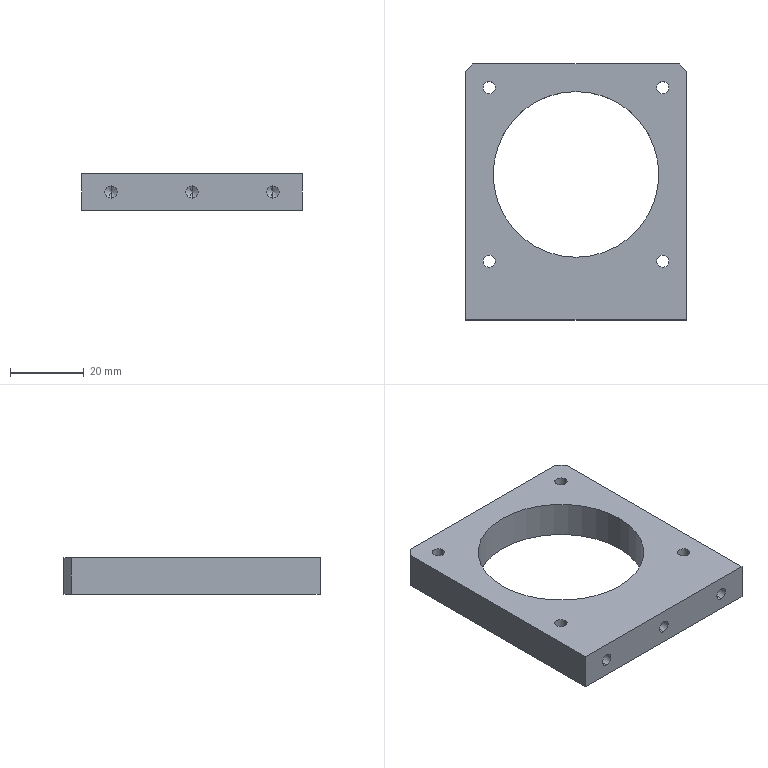Part | STEP file | 11-FG-B03711 | 1 solid | 38 faces | box 60 x 69.55 x 10 mm | volume 25100 mm3 | cylinder 20 | cone 10 | plane 8 | commonest cylinder face diameters 3.3 x14 2.5 x4 45 x2
STEP:
#1=CARTESIAN_POINT('',(-13.,22.5,3.5));
#2=VERTEX_POINT('',#1);
#3=CARTESIAN_POINT('',(-13.,22.5,6.));
#4=VERTEX_POINT('',#3);
#5=CARTESIAN_POINT('',(-13.,22.5,4.75));
#6=DIRECTION('',(0.,1.,0.));
#7=DIRECTION('',(0.,0.,1.));
#8=AXIS2_PLACEMENT_3D('',#5,#6,#7);
#9=CIRCLE('',#8,1.25);
#10=EDGE_CURVE('',#2,#4,#9,.T.);
#11=ORIENTED_EDGE('',*,*,#10,.F.);
#12=CARTESIAN_POINT('',(-13.,30.,3.5));
#13=VERTEX_POINT('',#12);
#14=CARTESIAN_POINT('',(-13.,30.,3.5));
#15=DIRECTION('',(0.,1.,0.));
#16=VECTOR('',#15,1000.);
#17=LINE('',#14,#16);
#18=EDGE_CURVE('',#2,#13,#17,.T.);
#19=ORIENTED_EDGE('',*,*,#18,.T.);
#20=CARTESIAN_POINT('',(-13.,30.,6.));
#21=VERTEX_POINT('',#20);
#22=CARTESIAN_POINT('',(-13.,30.,4.75));
#23=DIRECTION('',(0.,1.,0.));
#24=DIRECTION('',(0.,0.,1.));
#25=AXIS2_PLACEMENT_3D('',#22,#23,#24);
#26=CIRCLE('',#25,1.25);
#27=EDGE_CURVE('',#13,#21,#26,.T.);
#28=ORIENTED_EDGE('',*,*,#27,.T.);
#29=CARTESIAN_POINT('',(-13.,30.,6.));
#30=DIRECTION('',(0.,1.,0.));
#31=VECTOR('',#30,1000.);
#32=LINE('',#29,#31);
#33=EDGE_CURVE('',#4,#21,#32,.T.);
#34=ORIENTED_EDGE('',*,*,#33,.F.);
#35=EDGE_LOOP('',(#11,#19,#28,#34));
#36=FACE_OUTER_BOUND('',#35,.T.);
#37=CARTESIAN_POINT('',(-13.,30.,4.75));
#38=DIRECTION('',(0.,1.,0.));
#39=DIRECTION('',(0.,0.,1.));
#40=AXIS2_PLACEMENT_3D('',#37,#38,#39);
#41=CYLINDRICAL_SURFACE('',#40,1.25);
#42=ADVANCED_FACE('',(#36),#41,.F.);
#43=CARTESIAN_POINT('',(-13.,21.749,4.75));
#44=VERTEX_POINT('',#43);
#45=CARTESIAN_POINT('',(-13.,22.5,6.));
#46=DIRECTION('',(0.,0.515,0.8572));
#47=VECTOR('',#46,1000.);
#48=LINE('',#45,#47);
#49=EDGE_CURVE('',#44,#4,#48,.T.);
#50=ORIENTED_EDGE('',*,*,#49,.F.);
#51=CARTESIAN_POINT('',(-13.,22.5,3.5));
#52=DIRECTION('',(0.,0.515,-0.8572));
#53=VECTOR('',#52,1000.);
#54=LINE('',#51,#53);
#55=EDGE_CURVE('',#44,#2,#54,.T.);
#56=ORIENTED_EDGE('',*,*,#55,.T.);
#57=ORIENTED_EDGE('',*,*,#10,.T.);
#58=EDGE_LOOP('',(#50,#56,#57));
#59=FACE_OUTER_BOUND('',#58,.T.);
#60=CARTESIAN_POINT('',(-13.,22.5,4.75));
#61=DIRECTION('',(0.,1.,0.));
#62=DIRECTION('',(0.,0.,1.));
#63=AXIS2_PLACEMENT_3D('',#60,#61,#62);
#64=CONICAL_SURFACE('',#63,1.25,1.03);
#65=ADVANCED_FACE('',(#59),#64,.F.);
#66=CARTESIAN_POINT('',(14.,22.5,3.5));
#67=VERTEX_POINT('',#66);
#68=CARTESIAN_POINT('',(14.,22.5,6.));
#69=VERTEX_POINT('',#68);
#70=CARTESIAN_POINT('',(14.,22.5,4.75));
#71=DIRECTION('',(0.,1.,0.));
#72=DIRECTION('',(0.,0.,1.));
#73=AXIS2_PLACEMENT_3D('',#70,#71,#72);
#74=CIRCLE('',#73,1.25);
#75=EDGE_CURVE('',#67,#69,#74,.T.);
#76=ORIENTED_EDGE('',*,*,#75,.F.);
#77=CARTESIAN_POINT('',(14.,30.,3.5));
#78=VERTEX_POINT('',#77);
#79=CARTESIAN_POINT('',(14.,30.,3.5));
#80=DIRECTION('',(0.,1.,0.));
#81=VECTOR('',#80,1000.);
#82=LINE('',#79,#81);
#83=EDGE_CURVE('',#67,#78,#82,.T.);
#84=ORIENTED_EDGE('',*,*,#83,.T.);
#85=CARTESIAN_POINT('',(14.,30.,6.));
#86=VERTEX_POINT('',#85);
#87=CARTESIAN_POINT('',(14.,30.,4.75));
#88=DIRECTION('',(0.,1.,0.));
#89=DIRECTION('',(0.,0.,1.));
#90=AXIS2_PLACEMENT_3D('',#87,#88,#89);
#91=CIRCLE('',#90,1.25);
#92=EDGE_CURVE('',#78,#86,#91,.T.);
#93=ORIENTED_EDGE('',*,*,#92,.T.);
#94=CARTESIAN_POINT('',(14.,30.,6.));
#95=DIRECTION('',(0.,1.,0.));
#96=VECTOR('',#95,1000.);
#97=LINE('',#94,#96);
#98=EDGE_CURVE('',#69,#86,#97,.T.);
#99=ORIENTED_EDGE('',*,*,#98,.F.);
#100=EDGE_LOOP('',(#76,#84,#93,#99));
#101=FACE_OUTER_BOUND('',#100,.T.);
#102=CARTESIAN_POINT('',(14.,30.,4.75));
#103=DIRECTION('',(0.,1.,0.));
#104=DIRECTION('',(0.,0.,1.));
#105=AXIS2_PLACEMENT_3D('',#102,#103,#104);
#106=CYLINDRICAL_SURFACE('',#105,1.25);
#107=ADVANCED_FACE('',(#101),#106,.F.);
#108=CARTESIAN_POINT('',(14.,21.749,4.75));
#109=VERTEX_POINT('',#108);
#110=CARTESIAN_POINT('',(14.,22.5,6.));
#111=DIRECTION('',(0.,0.515,0.8572));
#112=VECTOR('',#111,1000.);
#113=LINE('',#110,#112);
#114=EDGE_CURVE('',#109,#69,#113,.T.);
#115=ORIENTED_EDGE('',*,*,#114,.F.);
#116=CARTESIAN_POINT('',(14.,22.5,3.5));
#117=DIRECTION('',(0.,0.515,-0.8572));
#118=VECTOR('',#117,1000.);
#119=LINE('',#116,#118);
#120=EDGE_CURVE('',#109,#67,#119,.T.);
#121=ORIENTED_EDGE('',*,*,#120,.T.);
#122=ORIENTED_EDGE('',*,*,#75,.T.);
#123=EDGE_LOOP('',(#115,#121,#122));
#124=FACE_OUTER_BOUND('',#123,.T.);
#125=CARTESIAN_POINT('',(14.,22.5,4.75));
#126=DIRECTION('',(0.,1.,0.));
#127=DIRECTION('',(0.,0.,1.));
#128=AXIS2_PLACEMENT_3D('',#125,#126,#127);
#129=CONICAL_SURFACE('',#128,1.25,1.03);
#130=ADVANCED_FACE('',(#124),#129,.F.);
#131=CARTESIAN_POINT('',(-22.,-29.45,6.65));
#132=VERTEX_POINT('',#131);
#133=CARTESIAN_POINT('',(-22.,-29.45,3.35));
#134=VERTEX_POINT('',#133);
#135=CARTESIAN_POINT('',(-22.,-29.45,5.));
#136=DIRECTION('',(0.,-1.,0.));
#137=DIRECTION('',(0.,0.,-1.));
#138=AXIS2_PLACEMENT_3D('',#135,#136,#137);
#139=CIRCLE('',#138,1.65);
#140=EDGE_CURVE('',#132,#134,#139,.T.);
#141=ORIENTED_EDGE('',*,*,#140,.F.);
#142=CARTESIAN_POINT('',(-22.,-39.55,6.65));
#143=VERTEX_POINT('',#142);
#144=CARTESIAN_POINT('',(-22.,-39.55,6.65));
#145=DIRECTION('',(0.,-1.,0.));
#146=VECTOR('',#145,1000.);
#147=LINE('',#144,#146);
#148=EDGE_CURVE('',#132,#143,#147,.T.);
#149=ORIENTED_EDGE('',*,*,#148,.T.);
#150=CARTESIAN_POINT('',(-22.,-39.55,3.35));
#151=VERTEX_POINT('',#150);
#152=CARTESIAN_POINT('',(-22.,-39.55,5.));
#153=DIRECTION('',(0.,-1.,0.));
#154=DIRECTION('',(0.,0.,-1.));
#155=AXIS2_PLACEMENT_3D('',#152,#153,#154);
#156=CIRCLE('',#155,1.65);
#157=EDGE_CURVE('',#143,#151,#156,.T.);
#158=ORIENTED_EDGE('',*,*,#157,.T.);
#159=CARTESIAN_POINT('',(-22.,-39.55,3.35));
#160=DIRECTION('',(0.,-1.,0.));
#161=VECTOR('',#160,1000.);
#162=LINE('',#159,#161);
#163=EDGE_CURVE('',#134,#151,#162,.T.);
#164=ORIENTED_EDGE('',*,*,#163,.F.);
#165=EDGE_LOOP('',(#141,#149,#158,#164));
#166=FACE_OUTER_BOUND('',#165,.T.);
#167=CARTESIAN_POINT('',(-22.,-39.55,5.));
#168=DIRECTION('',(0.,-1.,0.));
#169=DIRECTION('',(0.,0.,-1.));
#170=AXIS2_PLACEMENT_3D('',#167,#168,#169);
#171=CYLINDRICAL_SURFACE('',#170,1.65);
#172=ADVANCED_FACE('',(#166),#171,.F.);
#173=CARTESIAN_POINT('',(-22.,-28.459,5.));
#174=VERTEX_POINT('',#173);
#175=CARTESIAN_POINT('',(-22.,-29.45,3.35));
#176=DIRECTION('',(0.,-0.515,-0.8572));
#177=VECTOR('',#176,1000.);
#178=LINE('',#175,#177);
#179=EDGE_CURVE('',#174,#134,#178,.T.);
#180=ORIENTED_EDGE('',*,*,#179,.F.);
#181=CARTESIAN_POINT('',(-22.,-29.45,6.65));
#182=DIRECTION('',(0.,-0.515,0.8572));
#183=VECTOR('',#182,1000.);
#184=LINE('',#181,#183);
#185=EDGE_CURVE('',#174,#132,#184,.T.);
#186=ORIENTED_EDGE('',*,*,#185,.T.);
#187=ORIENTED_EDGE('',*,*,#140,.T.);
#188=EDGE_LOOP('',(#180,#186,#187));
#189=FACE_OUTER_BOUND('',#188,.T.);
#190=CARTESIAN_POINT('',(-22.,-29.45,5.));
#191=DIRECTION('',(0.,-1.,0.));
#192=DIRECTION('',(0.,0.,-1.));
#193=AXIS2_PLACEMENT_3D('',#190,#191,#192);
#194=CONICAL_SURFACE('',#193,1.65,1.03);
#195=ADVANCED_FACE('',(#189),#194,.F.);
#196=CARTESIAN_POINT('',(0.,-29.45,6.65));
#197=VERTEX_POINT('',#196);
#198=CARTESIAN_POINT('',(0.,-29.45,3.35));
#199=VERTEX_POINT('',#198);
#200=CARTESIAN_POINT('',(0.,-29.45,5.));
#201=DIRECTION('',(0.,-1.,0.));
#202=DIRECTION('',(0.,0.,-1.));
#203=AXIS2_PLACEMENT_3D('',#200,#201,#202);
#204=CIRCLE('',#203,1.65);
#205=EDGE_CURVE('',#197,#199,#204,.T.);
#206=ORIENTED_EDGE('',*,*,#205,.F.);
#207=CARTESIAN_POINT('',(0.,-39.55,6.65));
#208=VERTEX_POINT('',#207);
#209=CARTESIAN_POINT('',(0.,-39.55,6.65));
#210=DIRECTION('',(0.,-1.,0.));
#211=VECTOR('',#210,1000.);
#212=LINE('',#209,#211);
#213=EDGE_CURVE('',#197,#208,#212,.T.);
#214=ORIENTED_EDGE('',*,*,#213,.T.);
#215=CARTESIAN_POINT('',(0.,-39.55,3.35));
#216=VERTEX_POINT('',#215);
#217=CARTESIAN_POINT('',(0.,-39.55,5.));
#218=DIRECTION('',(0.,-1.,0.));
#219=DIRECTION('',(0.,0.,-1.));
#220=AXIS2_PLACEMENT_3D('',#217,#218,#219);
#221=CIRCLE('',#220,1.65);
#222=EDGE_CURVE('',#208,#216,#221,.T.);
#223=ORIENTED_EDGE('',*,*,#222,.T.);
#224=CARTESIAN_POINT('',(0.,-39.55,3.35));
#225=DIRECTION('',(0.,-1.,0.));
#226=VECTOR('',#225,1000.);
#227=LINE('',#224,#226);
#228=EDGE_CURVE('',#199,#216,#227,.T.);
#229=ORIENTED_EDGE('',*,*,#228,.F.);
#230=EDGE_LOOP('',(#206,#214,#223,#229));
#231=FACE_OUTER_BOUND('',#230,.T.);
#232=CARTESIAN_POINT('',(0.,-39.55,5.));
#233=DIRECTION('',(0.,-1.,0.));
#234=DIRECTION('',(0.,0.,-1.));
#235=AXIS2_PLACEMENT_3D('',#232,#233,#234);
#236=CYLINDRICAL_SURFACE('',#235,1.65);
#237=ADVANCED_FACE('',(#231),#236,.F.);
#238=CARTESIAN_POINT('',(0.,-28.459,5.));
#239=VERTEX_POINT('',#238);
#240=CARTESIAN_POINT('',(0.,-29.45,3.35));
#241=DIRECTION('',(0.,-0.515,-0.8572));
#242=VECTOR('',#241,1000.);
#243=LINE('',#240,#242);
#244=EDGE_CURVE('',#239,#199,#243,.T.);
#245=ORIENTED_EDGE('',*,*,#244,.F.);
#246=CARTESIAN_POINT('',(0.,-29.45,6.65));
#247=DIRECTION('',(0.,-0.515,0.8572));
#248=VECTOR('',#247,1000.);
#249=LINE('',#246,#248);
#250=EDGE_CURVE('',#239,#197,#249,.T.);
#251=ORIENTED_EDGE('',*,*,#250,.T.);
#252=ORIENTED_EDGE('',*,*,#205,.T.);
#253=EDGE_LOOP('',(#245,#251,#252));
#254=FACE_OUTER_BOUND('',#253,.T.);
#255=CARTESIAN_POINT('',(0.,-29.45,5.));
#256=DIRECTION('',(0.,-1.,0.));
#257=DIRECTION('',(0.,0.,-1.));
#258=AXIS2_PLACEMENT_3D('',#255,#256,#257);
#259=CONICAL_SURFACE('',#258,1.65,1.03);
#260=ADVANCED_FACE('',(#254),#259,.F.);
#261=CARTESIAN_POINT('',(22.,-29.45,6.65));
#262=VERTEX_POINT('',#261);
#263=CARTESIAN_POINT('',(22.,-29.45,3.35));
#264=VERTEX_POINT('',#263);
#265=CARTESIAN_POINT('',(22.,-29.45,5.));
#266=DIRECTION('',(0.,-1.,0.));
#267=DIRECTION('',(0.,0.,-1.));
#268=AXIS2_PLACEMENT_3D('',#265,#266,#267);
#269=CIRCLE('',#268,1.65);
#270=EDGE_CURVE('',#262,#264,#269,.T.);
#271=ORIENTED_EDGE('',*,*,#270,.F.);
#272=CARTESIAN_POINT('',(22.,-39.55,6.65));
#273=VERTEX_POINT('',#272);
#274=CARTESIAN_POINT('',(22.,-39.55,6.65));
#275=DIRECTION('',(0.,-1.,0.));
#276=VECTOR('',#275,1000.);
#277=LINE('',#274,#276);
#278=EDGE_CURVE('',#262,#273,#277,.T.);
#279=ORIENTED_EDGE('',*,*,#278,.T.);
#280=CARTESIAN_POINT('',(22.,-39.55,3.35));
#281=VERTEX_POINT('',#280);
#282=CARTESIAN_POINT('',(22.,-39.55,5.));
#283=DIRECTION('',(0.,-1.,0.));
#284=DIRECTION('',(0.,0.,-1.));
#285=AXIS2_PLACEMENT_3D('',#282,#283,#284);
#286=CIRCLE('',#285,1.65);
#287=EDGE_CURVE('',#273,#281,#286,.T.);
#288=ORIENTED_EDGE('',*,*,#287,.T.);
#289=CARTESIAN_POINT('',(22.,-39.55,3.35));
#290=DIRECTION('',(0.,-1.,0.));
#291=VECTOR('',#290,1000.);
#292=LINE('',#289,#291);
#293=EDGE_CURVE('',#264,#281,#292,.T.);
#294=ORIENTED_EDGE('',*,*,#293,.F.);
#295=EDGE_LOOP('',(#271,#279,#288,#294));
#296=FACE_OUTER_BOUND('',#295,.T.);
#297=CARTESIAN_POINT('',(22.,-39.55,5.));
#298=DIRECTION('',(0.,-1.,0.));
#299=DIRECTION('',(0.,0.,-1.));
#300=AXIS2_PLACEMENT_3D('',#297,#298,#299);
#301=CYLINDRICAL_SURFACE('',#300,1.65);
#302=ADVANCED_FACE('',(#296),#301,.F.);
#303=CARTESIAN_POINT('',(22.,-28.459,5.));
#304=VERTEX_POINT('',#303);
#305=CARTESIAN_POINT('',(22.,-29.45,3.35));
#306=DIRECTION('',(0.,-0.515,-0.8572));
#307=VECTOR('',#306,1000.);
#308=LINE('',#305,#307);
#309=EDGE_CURVE('',#304,#264,#308,.T.);
#310=ORIENTED_EDGE('',*,*,#309,.F.);
#311=CARTESIAN_POINT('',(22.,-29.45,6.65));
#312=DIRECTION('',(0.,-0.515,0.8572));
#313=VECTOR('',#312,1000.);
#314=LINE('',#311,#313);
#315=EDGE_CURVE('',#304,#262,#314,.T.);
#316=ORIENTED_EDGE('',*,*,#315,.T.);
#317=ORIENTED_EDGE('',*,*,#270,.T.);
#318=EDGE_LOOP('',(#310,#316,#317));
#319=FACE_OUTER_BOUND('',#318,.T.);
#320=CARTESIAN_POINT('',(22.,-29.45,5.));
#321=DIRECTION('',(0.,-1.,0.));
#322=DIRECTION('',(0.,0.,-1.));
#323=AXIS2_PLACEMENT_3D('',#320,#321,#322);
#324=CONICAL_SURFACE('',#323,1.65,1.03);
#325=ADVANCED_FACE('',(#319),#324,.F.);
#326=CARTESIAN_POINT('',(21.92,23.57,10.));
#327=VERTEX_POINT('',#326);
#328=CARTESIAN_POINT('',(25.22,23.57,10.));
#329=VERTEX_POINT('',#328);
#330=CARTESIAN_POINT('',(23.57,23.57,10.));
#331=DIRECTION('',(0.,0.,1.));
#332=DIRECTION('',(1.,0.,0.));
#333=AXIS2_PLACEMENT_3D('',#330,#331,#332);
#334=CIRCLE('',#333,1.65);
#335=EDGE_CURVE('',#327,#329,#334,.T.);
#336=ORIENTED_EDGE('',*,*,#335,.T.);
#337=CARTESIAN_POINT('',(25.22,23.57,0.));
#338=VERTEX_POINT('',#337);
#339=CARTESIAN_POINT('',(25.22,23.57,0.));
#340=DIRECTION('',(0.,0.,-1.));
#341=VECTOR('',#340,1000.);
#342=LINE('',#339,#341);
#343=EDGE_CURVE('',#329,#338,#342,.T.);
#344=ORIENTED_EDGE('',*,*,#343,.T.);
#345=CARTESIAN_POINT('',(21.92,23.57,0.));
#346=VERTEX_POINT('',#345);
#347=CARTESIAN_POINT('',(23.57,23.57,0.));
#348=DIRECTION('',(0.,0.,-1.));
#349=DIRECTION('',(-1.,0.,0.));
#350=AXIS2_PLACEMENT_3D('',#347,#348,#349);
#351=CIRCLE('',#350,1.65);
#352=EDGE_CURVE('',#338,#346,#351,.T.);
#353=ORIENTED_EDGE('',*,*,#352,.T.);
#354=CARTESIAN_POINT('',(21.92,23.57,0.));
#355=DIRECTION('',(0.,0.,-1.));
#356=VECTOR('',#355,1000.);
#357=LINE('',#354,#356);
#358=EDGE_CURVE('',#327,#346,#357,.T.);
#359=ORIENTED_EDGE('',*,*,#358,.F.);
#360=EDGE_LOOP('',(#336,#344,#353,#359));
#361=FACE_OUTER_BOUND('',#360,.T.);
#362=CARTESIAN_POINT('',(23.57,23.57,0.));
#363=DIRECTION('',(0.,0.,-1.));
#364=DIRECTION('',(-1.,0.,0.));
#365=AXIS2_PLACEMENT_3D('',#362,#363,#364);
#366=CYLINDRICAL_SURFACE('',#365,1.65);
#367=ADVANCED_FACE('',(#361),#366,.F.);
#368=CARTESIAN_POINT('',(21.92,-23.57,10.));
#369=VERTEX_POINT('',#368);
#370=CARTESIAN_POINT('',(25.22,-23.57,10.));
#371=VERTEX_POINT('',#370);
#372=CARTESIAN_POINT('',(23.57,-23.57,10.));
#373=DIRECTION('',(0.,0.,1.));
#374=DIRECTION('',(1.,0.,0.));
#375=AXIS2_PLACEMENT_3D('',#372,#373,#374);
#376=CIRCLE('',#375,1.65);
#377=EDGE_CURVE('',#369,#371,#376,.T.);
#378=ORIENTED_EDGE('',*,*,#377,.T.);
#379=CARTESIAN_POINT('',(25.22,-23.57,0.));
#380=VERTEX_POINT('',#379);
#381=CARTESIAN_POINT('',(25.22,-23.57,0.));
#382=DIRECTION('',(0.,0.,-1.));
#383=VECTOR('',#382,1000.);
#384=LINE('',#381,#383);
#385=EDGE_CURVE('',#371,#380,#384,.T.);
#386=ORIENTED_EDGE('',*,*,#385,.T.);
#387=CARTESIAN_POINT('',(21.92,-23.57,0.));
#388=VERTEX_POINT('',#387);
#389=CARTESIAN_POINT('',(23.57,-23.57,0.));
#390=DIRECTION('',(0.,0.,-1.));
#391=DIRECTION('',(-1.,0.,0.));
#392=AXIS2_PLACEMENT_3D('',#389,#390,#391);
#393=CIRCLE('',#392,1.65);
#394=EDGE_CURVE('',#380,#388,#393,.T.);
#395=ORIENTED_EDGE('',*,*,#394,.T.);
#396=CARTESIAN_POINT('',(21.92,-23.57,0.));
#397=DIRECTION('',(0.,0.,-1.));
#398=VECTOR('',#397,1000.);
#399=LINE('',#396,#398);
#400=EDGE_CURVE('',#369,#388,#399,.T.);
#401=ORIENTED_EDGE('',*,*,#400,.F.);
#402=EDGE_LOOP('',(#378,#386,#395,#401));
#403=FACE_OUTER_BOUND('',#402,.T.);
#404=CARTESIAN_POINT('',(23.57,-23.57,0.));
#405=DIRECTION('',(0.,0.,-1.));
#406=DIRECTION('',(-1.,0.,0.));
#407=AXIS2_PLACEMENT_3D('',#404,#405,#406);
#408=CYLINDRICAL_SURFACE('',#407,1.65);
#409=ADVANCED_FACE('',(#403),#408,.F.);
#410=CARTESIAN_POINT('',(-25.22,-23.57,10.));
#411=VERTEX_POINT('',#410);
#412=CARTESIAN_POINT('',(-21.92,-23.57,10.));
#413=VERTEX_POINT('',#412);
#414=CARTESIAN_POINT('',(-23.57,-23.57,10.));
#415=DIRECTION('',(0.,0.,1.));
#416=DIRECTION('',(1.,0.,0.));
#417=AXIS2_PLACEMENT_3D('',#414,#415,#416);
#418=CIRCLE('',#417,1.65);
#419=EDGE_CURVE('',#411,#413,#418,.T.);
#420=ORIENTED_EDGE('',*,*,#419,.T.);
#421=CARTESIAN_POINT('',(-21.92,-23.57,0.));
#422=VERTEX_POINT('',#421);
#423=CARTESIAN_POINT('',(-21.92,-23.57,0.));
#424=DIRECTION('',(0.,0.,-1.));
#425=VECTOR('',#424,1000.);
#426=LINE('',#423,#425);
#427=EDGE_CURVE('',#413,#422,#426,.T.);
#428=ORIENTED_EDGE('',*,*,#427,.T.);
#429=CARTESIAN_POINT('',(-25.22,-23.57,0.));
#430=VERTEX_POINT('',#429);
#431=CARTESIAN_POINT('',(-23.57,-23.57,0.));
#432=DIRECTION('',(0.,0.,-1.));
#433=DIRECTION('',(-1.,0.,0.));
#434=AXIS2_PLACEMENT_3D('',#431,#432,#433);
#435=CIRCLE('',#434,1.65);
#436=EDGE_CURVE('',#422,#430,#435,.T.);
#437=ORIENTED_EDGE('',*,*,#436,.T.);
#438=CARTESIAN_POINT('',(-25.22,-23.57,0.));
#439=DIRECTION('',(0.,0.,-1.));
#440=VECTOR('',#439,1000.);
#441=LINE('',#438,#440);
#442=EDGE_CURVE('',#411,#430,#441,.T.);
#443=ORIENTED_EDGE('',*,*,#442,.F.);
#444=EDGE_LOOP('',(#420,#428,#437,#443));
#445=FACE_OUTER_BOUND('',#444,.T.);
#446=CARTESIAN_POINT('',(-23.57,-23.57,0.));
#447=DIRECTION('',(0.,0.,-1.));
#448=DIRECTION('',(-1.,0.,0.));
#449=AXIS2_PLACEMENT_3D('',#446,#447,#448);
#450=CYLINDRICAL_SURFACE('',#449,1.65);
#451=ADVANCED_FACE('',(#445),#450,.F.);
#452=CARTESIAN_POINT('',(-25.22,23.57,10.));
#453=VERTEX_POINT('',#452);
#454=CARTESIAN_POINT('',(-21.92,23.57,10.));
#455=VERTEX_POINT('',#454);
#456=CARTESIAN_POINT('',(-23.57,23.57,10.));
#457=DIRECTION('',(0.,0.,1.));
#458=DIRECTION('',(1.,0.,0.));
#459=AXIS2_PLACEMENT_3D('',#456,#457,#458);
#460=CIRCLE('',#459,1.65);
#461=EDGE_CURVE('',#453,#455,#460,.T.);
#462=ORIENTED_EDGE('',*,*,#461,.T.);
#463=CARTESIAN_POINT('',(-21.92,23.57,0.));
#464=VERTEX_POINT('',#463);
#465=CARTESIAN_POINT('',(-21.92,23.57,0.));
#466=DIRECTION('',(0.,0.,-1.));
#467=VECTOR('',#466,1000.);
#468=LINE('',#465,#467);
#469=EDGE_CURVE('',#455,#464,#468,.T.);
#470=ORIENTED_EDGE('',*,*,#469,.T.);
#471=CARTESIAN_POINT('',(-25.22,23.57,0.));
#472=VERTEX_POINT('',#471);
#473=CARTESIAN_POINT('',(-23.57,23.57,0.));
#474=DIRECTION('',(0.,0.,-1.));
#475=DIRECTION('',(-1.,0.,0.));
#476=AXIS2_PLACEMENT_3D('',#473,#474,#475);
#477=CIRCLE('',#476,1.65);
#478=EDGE_CURVE('',#464,#472,#477,.T.);
#479=ORIENTED_EDGE('',*,*,#478,.T.);
#480=CARTESIAN_POINT('',(-25.22,23.57,0.));
#481=DIRECTION('',(0.,0.,-1.));
#482=VECTOR('',#481,1000.);
#483=LINE('',#480,#482);
#484=EDGE_CURVE('',#453,#472,#483,.T.);
#485=ORIENTED_EDGE('',*,*,#484,.F.);
#486=EDGE_LOOP('',(#462,#470,#479,#485));
#487=FACE_OUTER_BOUND('',#486,.T.);
#488=CARTESIAN_POINT('',(-23.57,23.57,0.));
#489=DIRECTION('',(0.,0.,-1.));
#490=DIRECTION('',(-1.,0.,0.));
#491=AXIS2_PLACEMENT_3D('',#488,#489,#490);
#492=CYLINDRICAL_SURFACE('',#491,1.65);
#493=ADVANCED_FACE('',(#487),#492,.F.);
#494=CARTESIAN_POINT('',(-22.5,0.,0.));
#495=VERTEX_POINT('',#494);
#496=CARTESIAN_POINT('',(22.5,0.,0.));
#497=VERTEX_POINT('',#496);
#498=CARTESIAN_POINT('',(0.,0.,0.));
#499=DIRECTION('',(0.,0.,1.));
#500=DIRECTION('',(1.,0.,0.));
#501=AXIS2_PLACEMENT_3D('',#498,#499,#500);
#502=CIRCLE('',#501,22.5);
#503=EDGE_CURVE('',#495,#497,#502,.T.);
#504=ORIENTED_EDGE('',*,*,#503,.F.);
#505=CARTESIAN_POINT('',(-22.5,0.,10.));
#506=VERTEX_POINT('',#505);
#507=CARTESIAN_POINT('',(-22.5,0.,-14.));
#508=DIRECTION('',(0.,0.,1.));
#509=VECTOR('',#508,1000.);
#510=LINE('',#507,#509);
#511=EDGE_CURVE('',#495,#506,#510,.T.);
#512=ORIENTED_EDGE('',*,*,#511,.T.);
#513=CARTESIAN_POINT('',(22.5,0.,10.));
#514=VERTEX_POINT('',#513);
#515=CARTESIAN_POINT('',(0.,0.,10.));
#516=DIRECTION('',(0.,0.,1.));
#517=DIRECTION('',(1.,0.,0.));
#518=AXIS2_PLACEMENT_3D('',#515,#516,#517);
#519=CIRCLE('',#518,22.5);
#520=EDGE_CURVE('',#506,#514,#519,.T.);
#521=ORIENTED_EDGE('',*,*,#520,.T.);
#522=CARTESIAN_POINT('',(22.5,0.,-14.));
#523=DIRECTION('',(0.,0.,1.));
#524=VECTOR('',#523,1000.);
#525=LINE('',#522,#524);
#526=EDGE_CURVE('',#497,#514,#525,.T.);
#527=ORIENTED_EDGE('',*,*,#526,.F.);
#528=EDGE_LOOP('',(#504,#512,#521,#527));
#529=FACE_OUTER_BOUND('',#528,.T.);
#530=CARTESIAN_POINT('',(0.,0.,-14.));
#531=DIRECTION('',(0.,0.,1.));
#532=DIRECTION('',(1.,0.,0.));
#533=AXIS2_PLACEMENT_3D('',#530,#531,#532);
#534=CYLINDRICAL_SURFACE('',#533,22.5);
#535=ADVANCED_FACE('',(#529),#534,.F.);
#536=CARTESIAN_POINT('',(30.,-39.55,0.));
#537=VERTEX_POINT('',#536);
#538=CARTESIAN_POINT('',(30.,28.,0.));
#539=VERTEX_POINT('',#538);
#540=CARTESIAN_POINT('',(30.,30.,0.));
#541=DIRECTION('',(0.,1.,0.));
#542=VECTOR('',#541,1000.);
#543=LINE('',#540,#542);
#544=EDGE_CURVE('',#537,#539,#543,.T.);
#545=ORIENTED_EDGE('',*,*,#544,.T.);
#546=CARTESIAN_POINT('',(30.,28.,10.));
#547=VERTEX_POINT('',#546);
#548=CARTESIAN_POINT('',(30.,28.,10.));
#549=DIRECTION('',(0.,0.,1.));
#550=VECTOR('',#549,1000.);
#551=LINE('',#548,#550);
#552=EDGE_CURVE('',#539,#547,#551,.T.);
#553=ORIENTED_EDGE('',*,*,#552,.T.);
#554=CARTESIAN_POINT('',(30.,-39.55,10.));
#555=VERTEX_POINT('',#554);
#556=CARTESIAN_POINT('',(30.,30.,10.));
#557=DIRECTION('',(0.,1.,0.));
#558=VECTOR('',#557,1000.);
#559=LINE('',#556,#558);
#560=EDGE_CURVE('',#555,#547,#559,.T.);
#561=ORIENTED_EDGE('',*,*,#560,.F.);
#562=CARTESIAN_POINT('',(30.,-39.55,70.755));
#563=DIRECTION('',(0.,0.,-1.));
#564=VECTOR('',#563,1000.);
#565=LINE('',#562,#564);
#566=EDGE_CURVE('',#555,#537,#565,.T.);
#567=ORIENTED_EDGE('',*,*,#566,.T.);
#568=EDGE_LOOP('',(#545,#553,#561,#567));
#569=FACE_OUTER_BOUND('',#568,.T.);
#570=CARTESIAN_POINT('',(30.,30.,10.));
#571=DIRECTION('',(-1.,0.,0.));
#572=DIRECTION('',(0.,-1.,0.));
#573=AXIS2_PLACEMENT_3D('',#570,#571,#572);
#574=PLANE('',#573);
#575=ADVANCED_FACE('',(#569),#574,.F.);
#576=CARTESIAN_POINT('',(-13.,30.,4.75));
#577=DIRECTION('',(0.,1.,0.));
#578=DIRECTION('',(0.,0.,1.));
#579=AXIS2_PLACEMENT_3D('',#576,#577,#578);
#580=CIRCLE('',#579,1.25);
#581=EDGE_CURVE('',#21,#13,#580,.T.);
#582=ORIENTED_EDGE('',*,*,#581,.F.);
#583=ORIENTED_EDGE('',*,*,#27,.F.);
#584=EDGE_LOOP('',(#582,#583));
#585=FACE_BOUND('',#584,.T.);
#586=CARTESIAN_POINT('',(14.,30.,4.75));
#587=DIRECTION('',(0.,1.,0.));
#588=DIRECTION('',(0.,0.,1.));
#589=AXIS2_PLACEMENT_3D('',#586,#587,#588);
#590=CIRCLE('',#589,1.25);
#591=EDGE_CURVE('',#86,#78,#590,.T.);
#592=ORIENTED_EDGE('',*,*,#591,.F.);
#593=ORIENTED_EDGE('',*,*,#92,.F.);
#594=EDGE_LOOP('',(#592,#593));
#595=FACE_BOUND('',#594,.T.);
#596=CARTESIAN_POINT('',(28.,30.,10.));
#597=VERTEX_POINT('',#596);
#598=CARTESIAN_POINT('',(-28.,30.,10.));
#599=VERTEX_POINT('',#598);
#600=CARTESIAN_POINT('',(-30.,30.,10.));
#601=DIRECTION('',(-1.,0.,0.));
#602=VECTOR('',#601,1000.);
#603=LINE('',#600,#602);
#604=EDGE_CURVE('',#597,#599,#603,.T.);
#605=ORIENTED_EDGE('',*,*,#604,.F.);
#606=CARTESIAN_POINT('',(28.,30.,0.));
#607=VERTEX_POINT('',#606);
#608=CARTESIAN_POINT('',(28.,30.,10.));
#609=DIRECTION('',(0.,0.,-1.));
#610=VECTOR('',#609,1000.);
#611=LINE('',#608,#610);
#612=EDGE_CURVE('',#597,#607,#611,.T.);
#613=ORIENTED_EDGE('',*,*,#612,.T.);
#614=CARTESIAN_POINT('',(-28.,30.,0.));
#615=VERTEX_POINT('',#614);
#616=CARTESIAN_POINT('',(-30.,30.,0.));
#617=DIRECTION('',(-1.,0.,0.));
#618=VECTOR('',#617,1000.);
#619=LINE('',#616,#618);
#620=EDGE_CURVE('',#607,#615,#619,.T.);
#621=ORIENTED_EDGE('',*,*,#620,.T.);
#622=CARTESIAN_POINT('',(-28.,30.,10.));
#623=DIRECTION('',(0.,0.,1.));
#624=VECTOR('',#623,1000.);
#625=LINE('',#622,#624);
#626=EDGE_CURVE('',#615,#599,#625,.T.);
#627=ORIENTED_EDGE('',*,*,#626,.T.);
#628=EDGE_LOOP('',(#605,#613,#621,#627));
#629=FACE_OUTER_BOUND('',#628,.T.);
#630=CARTESIAN_POINT('',(-30.,30.,10.));
#631=DIRECTION('',(0.,-1.,0.));
#632=DIRECTION('',(0.,0.,-1.));
#633=AXIS2_PLACEMENT_3D('',#630,#631,#632);
#634=PLANE('',#633);
#635=ADVANCED_FACE('',(#585,#595,#629),#634,.F.);
#636=CARTESIAN_POINT('',(-30.,28.,10.));
#637=VERTEX_POINT('',#636);
#638=CARTESIAN_POINT('',(-30.,-39.55,10.));
#639=VERTEX_POINT('',#638);
#640=CARTESIAN_POINT('',(-30.,30.,10.));
#641=DIRECTION('',(0.,-1.,0.));
#642=VECTOR('',#641,1000.);
#643=LINE('',#640,#642);
#644=EDGE_CURVE('',#637,#639,#643,.T.);
#645=ORIENTED_EDGE('',*,*,#644,.F.);
#646=CARTESIAN_POINT('',(-30.,28.,0.));
#647=VERTEX_POINT('',#646);
#648=CARTESIAN_POINT('',(-30.,28.,10.));
#649=DIRECTION('',(0.,0.,-1.));
#650=VECTOR('',#649,1000.);
#651=LINE('',#648,#650);
#652=EDGE_CURVE('',#637,#647,#651,.T.);
#653=ORIENTED_EDGE('',*,*,#652,.T.);
#654=CARTESIAN_POINT('',(-30.,-39.55,0.));
#655=VERTEX_POINT('',#654);
#656=CARTESIAN_POINT('',(-30.,30.,0.));
#657=DIRECTION('',(0.,-1.,0.));
#658=VECTOR('',#657,1000.);
#659=LINE('',#656,#658);
#660=EDGE_CURVE('',#647,#655,#659,.T.);
#661=ORIENTED_EDGE('',*,*,#660,.T.);
#662=CARTESIAN_POINT('',(-30.,-39.55,70.755));
#663=DIRECTION('',(0.,0.,-1.));
#664=VECTOR('',#663,1000.);
#665=LINE('',#662,#664);
#666=EDGE_CURVE('',#639,#655,#665,.T.);
#667=ORIENTED_EDGE('',*,*,#666,.F.);
#668=EDGE_LOOP('',(#645,#653,#661,#667));
#669=FACE_OUTER_BOUND('',#668,.T.);
#670=CARTESIAN_POINT('',(-30.,30.,10.));
#671=DIRECTION('',(1.,0.,0.));
#672=DIRECTION('',(0.,1.,0.));
#673=AXIS2_PLACEMENT_3D('',#670,#671,#672);
#674=PLANE('',#673);
#675=ADVANCED_FACE('',(#669),#674,.F.);
#676=ORIENTED_EDGE('',*,*,#335,.F.);
#677=CARTESIAN_POINT('',(23.57,23.57,10.));
#678=DIRECTION('',(0.,0.,1.));
#679=DIRECTION('',(1.,0.,0.));
#680=AXIS2_PLACEMENT_3D('',#677,#678,#679);
#681=CIRCLE('',#680,1.65);
#682=EDGE_CURVE('',#329,#327,#681,.T.);
#683=ORIENTED_EDGE('',*,*,#682,.F.);
#684=EDGE_LOOP('',(#676,#683));
#685=FACE_BOUND('',#684,.T.);
#686=ORIENTED_EDGE('',*,*,#377,.F.);
#687=CARTESIAN_POINT('',(23.57,-23.57,10.));
#688=DIRECTION('',(0.,0.,1.));
#689=DIRECTION('',(1.,0.,0.));
#690=AXIS2_PLACEMENT_3D('',#687,#688,#689);
#691=CIRCLE('',#690,1.65);
#692=EDGE_CURVE('',#371,#369,#691,.T.);
#693=ORIENTED_EDGE('',*,*,#692,.F.);
#694=EDGE_LOOP('',(#686,#693));
#695=FACE_BOUND('',#694,.T.);
#696=ORIENTED_EDGE('',*,*,#419,.F.);
#697=CARTESIAN_POINT('',(-23.57,-23.57,10.));
#698=DIRECTION('',(0.,0.,1.));
#699=DIRECTION('',(1.,0.,0.));
#700=AXIS2_PLACEMENT_3D('',#697,#698,#699);
#701=CIRCLE('',#700,1.65);
#702=EDGE_CURVE('',#413,#411,#701,.T.);
#703=ORIENTED_EDGE('',*,*,#702,.F.);
#704=EDGE_LOOP('',(#696,#703));
#705=FACE_BOUND('',#704,.T.);
#706=ORIENTED_EDGE('',*,*,#461,.F.);
#707=CARTESIAN_POINT('',(-23.57,23.57,10.));
#708=DIRECTION('',(0.,0.,1.));
#709=DIRECTION('',(1.,0.,0.));
#710=AXIS2_PLACEMENT_3D('',#707,#708,#709);
#711=CIRCLE('',#710,1.65);
#712=EDGE_CURVE('',#455,#453,#711,.T.);
#713=ORIENTED_EDGE('',*,*,#712,.F.);
#714=EDGE_LOOP('',(#706,#713));
#715=FACE_BOUND('',#714,.T.);
#716=CARTESIAN_POINT('',(0.,0.,10.));
#717=DIRECTION('',(0.,0.,1.));
#718=DIRECTION('',(1.,0.,0.));
#719=AXIS2_PLACEMENT_3D('',#716,#717,#718);
#720=CIRCLE('',#719,22.5);
#721=EDGE_CURVE('',#514,#506,#720,.T.);
#722=ORIENTED_EDGE('',*,*,#721,.F.);
#723=ORIENTED_EDGE('',*,*,#520,.F.);
#724=EDGE_LOOP('',(#722,#723));
#725=FACE_BOUND('',#724,.T.);
#726=ORIENTED_EDGE('',*,*,#560,.T.);
#727=CARTESIAN_POINT('',(29.,29.,10.));
#728=DIRECTION('',(-0.7071,0.7071,0.));
#729=VECTOR('',#728,1000.);
#730=LINE('',#727,#729);
#731=EDGE_CURVE('',#547,#597,#730,.T.);
#732=ORIENTED_EDGE('',*,*,#731,.T.);
#733=ORIENTED_EDGE('',*,*,#604,.T.);
#734=CARTESIAN_POINT('',(-29.,29.,10.));
#735=DIRECTION('',(-0.7071,-0.7071,0.));
#736=VECTOR('',#735,1000.);
#737=LINE('',#734,#736);
#738=EDGE_CURVE('',#599,#637,#737,.T.);
#739=ORIENTED_EDGE('',*,*,#738,.T.);
#740=ORIENTED_EDGE('',*,*,#644,.T.);
#741=CARTESIAN_POINT('',(30.,-39.55,10.));
#742=DIRECTION('',(-1.,0.,0.));
#743=VECTOR('',#742,1000.);
#744=LINE('',#741,#743);
#745=EDGE_CURVE('',#555,#639,#744,.T.);
#746=ORIENTED_EDGE('',*,*,#745,.F.);
#747=EDGE_LOOP('',(#726,#732,#733,#739,#740,#746));
#748=FACE_OUTER_BOUND('',#747,.T.);
#749=CARTESIAN_POINT('',(0.,0.,10.));
#750=DIRECTION('',(0.,0.,1.));
#751=DIRECTION('',(1.,0.,0.));
#752=AXIS2_PLACEMENT_3D('',#749,#750,#751);
#753=PLANE('',#752);
#754=ADVANCED_FACE('',(#685,#695,#705,#715,#725,#748),#753,.T.);
#755=CARTESIAN_POINT('',(23.57,23.57,0.));
#756=DIRECTION('',(0.,0.,-1.));
#757=DIRECTION('',(-1.,0.,0.));
#758=AXIS2_PLACEMENT_3D('',#755,#756,#757);
#759=CIRCLE('',#758,1.65);
#760=EDGE_CURVE('',#346,#338,#759,.T.);
#761=ORIENTED_EDGE('',*,*,#760,.F.);
#762=ORIENTED_EDGE('',*,*,#352,.F.);
#763=EDGE_LOOP('',(#761,#762));
#764=FACE_BOUND('',#763,.T.);
#765=CARTESIAN_POINT('',(23.57,-23.57,0.));
#766=DIRECTION('',(0.,0.,-1.));
#767=DIRECTION('',(-1.,0.,0.));
#768=AXIS2_PLACEMENT_3D('',#765,#766,#767);
#769=CIRCLE('',#768,1.65);
#770=EDGE_CURVE('',#388,#380,#769,.T.);
#771=ORIENTED_EDGE('',*,*,#770,.F.);
#772=ORIENTED_EDGE('',*,*,#394,.F.);
#773=EDGE_LOOP('',(#771,#772));
#774=FACE_BOUND('',#773,.T.);
#775=CARTESIAN_POINT('',(-23.57,-23.57,0.));
#776=DIRECTION('',(0.,0.,-1.));
#777=DIRECTION('',(-1.,0.,0.));
#778=AXIS2_PLACEMENT_3D('',#775,#776,#777);
#779=CIRCLE('',#778,1.65);
#780=EDGE_CURVE('',#430,#422,#779,.T.);
#781=ORIENTED_EDGE('',*,*,#780,.F.);
#782=ORIENTED_EDGE('',*,*,#436,.F.);
#783=EDGE_LOOP('',(#781,#782));
#784=FACE_BOUND('',#783,.T.);
#785=CARTESIAN_POINT('',(-23.57,23.57,0.));
#786=DIRECTION('',(0.,0.,-1.));
#787=DIRECTION('',(-1.,0.,0.));
#788=AXIS2_PLACEMENT_3D('',#785,#786,#787);
#789=CIRCLE('',#788,1.65);
#790=EDGE_CURVE('',#472,#464,#789,.T.);
#791=ORIENTED_EDGE('',*,*,#790,.F.);
#792=ORIENTED_EDGE('',*,*,#478,.F.);
#793=EDGE_LOOP('',(#791,#792));
#794=FACE_BOUND('',#793,.T.);
#795=CARTESIAN_POINT('',(0.,0.,0.));
#796=DIRECTION('',(0.,0.,1.));
#797=DIRECTION('',(1.,0.,0.));
#798=AXIS2_PLACEMENT_3D('',#795,#796,#797);
#799=CIRCLE('',#798,22.5);
#800=EDGE_CURVE('',#497,#495,#799,.T.);
#801=ORIENTED_EDGE('',*,*,#800,.T.);
#802=ORIENTED_EDGE('',*,*,#503,.T.);
#803=EDGE_LOOP('',(#801,#802));
#804=FACE_BOUND('',#803,.T.);
#805=ORIENTED_EDGE('',*,*,#620,.F.);
#806=CARTESIAN_POINT('',(28.,30.,0.));
#807=DIRECTION('',(0.7071,-0.7071,0.));
#808=VECTOR('',#807,1000.);
#809=LINE('',#806,#808);
#810=EDGE_CURVE('',#607,#539,#809,.T.);
#811=ORIENTED_EDGE('',*,*,#810,.T.);
#812=ORIENTED_EDGE('',*,*,#544,.F.);
#813=CARTESIAN_POINT('',(30.,-39.55,0.));
#814=DIRECTION('',(-1.,0.,0.));
#815=VECTOR('',#814,1000.);
#816=LINE('',#813,#815);
#817=EDGE_CURVE('',#537,#655,#816,.T.);
#818=ORIENTED_EDGE('',*,*,#817,.T.);
#819=ORIENTED_EDGE('',*,*,#660,.F.);
#820=CARTESIAN_POINT('',(-30.,28.,0.));
#821=DIRECTION('',(0.7071,0.7071,0.));
#822=VECTOR('',#821,1000.);
#823=LINE('',#820,#822);
#824=EDGE_CURVE('',#647,#615,#823,.T.);
#825=ORIENTED_EDGE('',*,*,#824,.T.);
#826=EDGE_LOOP('',(#805,#811,#812,#818,#819,#825));
#827=FACE_OUTER_BOUND('',#826,.T.);
#828=CARTESIAN_POINT('',(0.,0.,0.));
#829=DIRECTION('',(0.,0.,1.));
#830=DIRECTION('',(1.,0.,0.));
#831=AXIS2_PLACEMENT_3D('',#828,#829,#830);
#832=PLANE('',#831);
#833=ADVANCED_FACE('',(#764,#774,#784,#794,#804,#827),#832,.F.);
#834=ORIENTED_EDGE('',*,*,#511,.F.);
#835=ORIENTED_EDGE('',*,*,#800,.F.);
#836=ORIENTED_EDGE('',*,*,#526,.T.);
#837=ORIENTED_EDGE('',*,*,#721,.T.);
#838=EDGE_LOOP('',(#834,#835,#836,#837));
#839=FACE_OUTER_BOUND('',#838,.T.);
#840=CARTESIAN_POINT('',(0.,0.,-14.));
#841=DIRECTION('',(0.,0.,1.));
#842=DIRECTION('',(1.,0.,0.));
#843=AXIS2_PLACEMENT_3D('',#840,#841,#842);
#844=CYLINDRICAL_SURFACE('',#843,22.5);
#845=ADVANCED_FACE('',(#839),#844,.F.);
#846=ORIENTED_EDGE('',*,*,#469,.F.);
#847=ORIENTED_EDGE('',*,*,#712,.T.);
#848=ORIENTED_EDGE('',*,*,#484,.T.);
#849=ORIENTED_EDGE('',*,*,#790,.T.);
#850=EDGE_LOOP('',(#846,#847,#848,#849));
#851=FACE_OUTER_BOUND('',#850,.T.);
#852=CARTESIAN_POINT('',(-23.57,23.57,0.));
#853=DIRECTION('',(0.,0.,-1.));
#854=DIRECTION('',(-1.,0.,0.));
#855=AXIS2_PLACEMENT_3D('',#852,#853,#854);
#856=CYLINDRICAL_SURFACE('',#855,1.65);
#857=ADVANCED_FACE('',(#851),#856,.F.);
#858=ORIENTED_EDGE('',*,*,#427,.F.);
#859=ORIENTED_EDGE('',*,*,#702,.T.);
#860=ORIENTED_EDGE('',*,*,#442,.T.);
#861=ORIENTED_EDGE('',*,*,#780,.T.);
#862=EDGE_LOOP('',(#858,#859,#860,#861));
#863=FACE_OUTER_BOUND('',#862,.T.);
#864=CARTESIAN_POINT('',(-23.57,-23.57,0.));
#865=DIRECTION('',(0.,0.,-1.));
#866=DIRECTION('',(-1.,0.,0.));
#867=AXIS2_PLACEMENT_3D('',#864,#865,#866);
#868=CYLINDRICAL_SURFACE('',#867,1.65);
#869=ADVANCED_FACE('',(#863),#868,.F.);
#870=ORIENTED_EDGE('',*,*,#385,.F.);
#871=ORIENTED_EDGE('',*,*,#692,.T.);
#872=ORIENTED_EDGE('',*,*,#400,.T.);
#873=ORIENTED_EDGE('',*,*,#770,.T.);
#874=EDGE_LOOP('',(#870,#871,#872,#873));
#875=FACE_OUTER_BOUND('',#874,.T.);
#876=CARTESIAN_POINT('',(23.57,-23.57,0.));
#877=DIRECTION('',(0.,0.,-1.));
#878=DIRECTION('',(-1.,0.,0.));
#879=AXIS2_PLACEMENT_3D('',#876,#877,#878);
#880=CYLINDRICAL_SURFACE('',#879,1.65);
#881=ADVANCED_FACE('',(#875),#880,.F.);
#882=ORIENTED_EDGE('',*,*,#343,.F.);
#883=ORIENTED_EDGE('',*,*,#682,.T.);
#884=ORIENTED_EDGE('',*,*,#358,.T.);
#885=ORIENTED_EDGE('',*,*,#760,.T.);
#886=EDGE_LOOP('',(#882,#883,#884,#885));
#887=FACE_OUTER_BOUND('',#886,.T.);
#888=CARTESIAN_POINT('',(23.57,23.57,0.));
#889=DIRECTION('',(0.,0.,-1.));
#890=DIRECTION('',(-1.,0.,0.));
#891=AXIS2_PLACEMENT_3D('',#888,#889,#890);
#892=CYLINDRICAL_SURFACE('',#891,1.65);
#893=ADVANCED_FACE('',(#887),#892,.F.);
#894=CARTESIAN_POINT('',(-22.,-39.55,5.));
#895=DIRECTION('',(0.,-1.,0.));
#896=DIRECTION('',(0.,0.,-1.));
#897=AXIS2_PLACEMENT_3D('',#894,#895,#896);
#898=CIRCLE('',#897,1.65);
#899=EDGE_CURVE('',#151,#143,#898,.T.);
#900=ORIENTED_EDGE('',*,*,#899,.F.);
#901=ORIENTED_EDGE('',*,*,#157,.F.);
#902=EDGE_LOOP('',(#900,#901));
#903=FACE_BOUND('',#902,.T.);
#904=CARTESIAN_POINT('',(0.,-39.55,5.));
#905=DIRECTION('',(0.,-1.,0.));
#906=DIRECTION('',(0.,0.,-1.));
#907=AXIS2_PLACEMENT_3D('',#904,#905,#906);
#908=CIRCLE('',#907,1.65);
#909=EDGE_CURVE('',#216,#208,#908,.T.);
#910=ORIENTED_EDGE('',*,*,#909,.F.);
#911=ORIENTED_EDGE('',*,*,#222,.F.);
#912=EDGE_LOOP('',(#910,#911));
#913=FACE_BOUND('',#912,.T.);
#914=CARTESIAN_POINT('',(22.,-39.55,5.));
#915=DIRECTION('',(0.,-1.,0.));
#916=DIRECTION('',(0.,0.,-1.));
#917=AXIS2_PLACEMENT_3D('',#914,#915,#916);
#918=CIRCLE('',#917,1.65);
#919=EDGE_CURVE('',#281,#273,#918,.T.);
#920=ORIENTED_EDGE('',*,*,#919,.F.);
#921=ORIENTED_EDGE('',*,*,#287,.F.);
#922=EDGE_LOOP('',(#920,#921));
#923=FACE_BOUND('',#922,.T.);
#924=ORIENTED_EDGE('',*,*,#566,.F.);
#925=ORIENTED_EDGE('',*,*,#745,.T.);
#926=ORIENTED_EDGE('',*,*,#666,.T.);
#927=ORIENTED_EDGE('',*,*,#817,.F.);
#928=EDGE_LOOP('',(#924,#925,#926,#927));
#929=FACE_OUTER_BOUND('',#928,.T.);
#930=CARTESIAN_POINT('',(30.,-39.55,70.755));
#931=DIRECTION('',(0.,-1.,0.));
#932=DIRECTION('',(0.,0.,-1.));
#933=AXIS2_PLACEMENT_3D('',#930,#931,#932);
#934=PLANE('',#933);
#935=ADVANCED_FACE('',(#903,#913,#923,#929),#934,.T.);
#936=ORIENTED_EDGE('',*,*,#731,.F.);
#937=ORIENTED_EDGE('',*,*,#552,.F.);
#938=ORIENTED_EDGE('',*,*,#810,.F.);
#939=ORIENTED_EDGE('',*,*,#612,.F.);
#940=EDGE_LOOP('',(#936,#937,#938,#939));
#941=FACE_OUTER_BOUND('',#940,.T.);
#942=CARTESIAN_POINT('',(28.,30.,10.));
#943=DIRECTION('',(-0.7071,-0.7071,0.));
#944=DIRECTION('',(0.,0.,-1.));
#945=AXIS2_PLACEMENT_3D('',#942,#943,#944);
#946=PLANE('',#945);
#947=ADVANCED_FACE('',(#941),#946,.F.);
#948=ORIENTED_EDGE('',*,*,#738,.F.);
#949=ORIENTED_EDGE('',*,*,#626,.F.);
#950=ORIENTED_EDGE('',*,*,#824,.F.);
#951=ORIENTED_EDGE('',*,*,#652,.F.);
#952=EDGE_LOOP('',(#948,#949,#950,#951));
#953=FACE_OUTER_BOUND('',#952,.T.);
#954=CARTESIAN_POINT('',(-30.,28.,10.));
#955=DIRECTION('',(0.7071,-0.7071,0.));
#956=DIRECTION('',(0.,0.,-1.));
#957=AXIS2_PLACEMENT_3D('',#954,#955,#956);
#958=PLANE('',#957);
#959=ADVANCED_FACE('',(#953),#958,.F.);
#960=ORIENTED_EDGE('',*,*,#315,.F.);
#961=ORIENTED_EDGE('',*,*,#309,.T.);
#962=CARTESIAN_POINT('',(22.,-29.45,5.));
#963=DIRECTION('',(0.,-1.,0.));
#964=DIRECTION('',(0.,0.,-1.));
#965=AXIS2_PLACEMENT_3D('',#962,#963,#964);
#966=CIRCLE('',#965,1.65);
#967=EDGE_CURVE('',#264,#262,#966,.T.);
#968=ORIENTED_EDGE('',*,*,#967,.T.);
#969=EDGE_LOOP('',(#960,#961,#968));
#970=FACE_OUTER_BOUND('',#969,.T.);
#971=CARTESIAN_POINT('',(22.,-29.45,5.));
#972=DIRECTION('',(0.,-1.,0.));
#973=DIRECTION('',(0.,0.,-1.));
#974=AXIS2_PLACEMENT_3D('',#971,#972,#973);
#975=CONICAL_SURFACE('',#974,1.65,1.03);
#976=ADVANCED_FACE('',(#970),#975,.F.);
#977=ORIENTED_EDGE('',*,*,#278,.F.);
#978=ORIENTED_EDGE('',*,*,#967,.F.);
#979=ORIENTED_EDGE('',*,*,#293,.T.);
#980=ORIENTED_EDGE('',*,*,#919,.T.);
#981=EDGE_LOOP('',(#977,#978,#979,#980));
#982=FACE_OUTER_BOUND('',#981,.T.);
#983=CARTESIAN_POINT('',(22.,-39.55,5.));
#984=DIRECTION('',(0.,-1.,0.));
#985=DIRECTION('',(0.,0.,-1.));
#986=AXIS2_PLACEMENT_3D('',#983,#984,#985);
#987=CYLINDRICAL_SURFACE('',#986,1.65);
#988=ADVANCED_FACE('',(#982),#987,.F.);
#989=ORIENTED_EDGE('',*,*,#250,.F.);
#990=ORIENTED_EDGE('',*,*,#244,.T.);
#991=CARTESIAN_POINT('',(0.,-29.45,5.));
#992=DIRECTION('',(0.,-1.,0.));
#993=DIRECTION('',(0.,0.,-1.));
#994=AXIS2_PLACEMENT_3D('',#991,#992,#993);
#995=CIRCLE('',#994,1.65);
#996=EDGE_CURVE('',#199,#197,#995,.T.);
#997=ORIENTED_EDGE('',*,*,#996,.T.);
#998=EDGE_LOOP('',(#989,#990,#997));
#999=FACE_OUTER_BOUND('',#998,.T.);
#1000=CARTESIAN_POINT('',(0.,-29.45,5.));
#1001=DIRECTION('',(0.,-1.,0.));
#1002=DIRECTION('',(0.,0.,-1.));
#1003=AXIS2_PLACEMENT_3D('',#1000,#1001,#1002);
#1004=CONICAL_SURFACE('',#1003,1.65,1.03);
#1005=ADVANCED_FACE('',(#999),#1004,.F.);
#1006=ORIENTED_EDGE('',*,*,#213,.F.);
#1007=ORIENTED_EDGE('',*,*,#996,.F.);
#1008=ORIENTED_EDGE('',*,*,#228,.T.);
#1009=ORIENTED_EDGE('',*,*,#909,.T.);
#1010=EDGE_LOOP('',(#1006,#1007,#1008,#1009));
#1011=FACE_OUTER_BOUND('',#1010,.T.);
#1012=CARTESIAN_POINT('',(0.,-39.55,5.));
#1013=DIRECTION('',(0.,-1.,0.));
#1014=DIRECTION('',(0.,0.,-1.));
#1015=AXIS2_PLACEMENT_3D('',#1012,#1013,#1014);
#1016=CYLINDRICAL_SURFACE('',#1015,1.65);
#1017=ADVANCED_FACE('',(#1011),#1016,.F.);
#1018=ORIENTED_EDGE('',*,*,#185,.F.);
#1019=ORIENTED_EDGE('',*,*,#179,.T.);
#1020=CARTESIAN_POINT('',(-22.,-29.45,5.));
#1021=DIRECTION('',(0.,-1.,0.));
#1022=DIRECTION('',(0.,0.,-1.));
#1023=AXIS2_PLACEMENT_3D('',#1020,#1021,#1022);
#1024=CIRCLE('',#1023,1.65);
#1025=EDGE_CURVE('',#134,#132,#1024,.T.);
#1026=ORIENTED_EDGE('',*,*,#1025,.T.);
#1027=EDGE_LOOP('',(#1018,#1019,#1026));
#1028=FACE_OUTER_BOUND('',#1027,.T.);
#1029=CARTESIAN_POINT('',(-22.,-29.45,5.));
#1030=DIRECTION('',(0.,-1.,0.));
#1031=DIRECTION('',(0.,0.,-1.));
#1032=AXIS2_PLACEMENT_3D('',#1029,#1030,#1031);
#1033=CONICAL_SURFACE('',#1032,1.65,1.03);
#1034=ADVANCED_FACE('',(#1028),#1033,.F.);
#1035=ORIENTED_EDGE('',*,*,#148,.F.);
#1036=ORIENTED_EDGE('',*,*,#1025,.F.);
#1037=ORIENTED_EDGE('',*,*,#163,.T.);
#1038=ORIENTED_EDGE('',*,*,#899,.T.);
#1039=EDGE_LOOP('',(#1035,#1036,#1037,#1038));
#1040=FACE_OUTER_BOUND('',#1039,.T.);
#1041=CARTESIAN_POINT('',(-22.,-39.55,5.));
#1042=DIRECTION('',(0.,-1.,0.));
#1043=DIRECTION('',(0.,0.,-1.));
#1044=AXIS2_PLACEMENT_3D('',#1041,#1042,#1043);
#1045=CYLINDRICAL_SURFACE('',#1044,1.65);
#1046=ADVANCED_FACE('',(#1040),#1045,.F.);
#1047=ORIENTED_EDGE('',*,*,#120,.F.);
#1048=ORIENTED_EDGE('',*,*,#114,.T.);
#1049=CARTESIAN_POINT('',(14.,22.5,4.75));
#1050=DIRECTION('',(0.,1.,0.));
#1051=DIRECTION('',(0.,0.,1.));
#1052=AXIS2_PLACEMENT_3D('',#1049,#1050,#1051);
#1053=CIRCLE('',#1052,1.25);
#1054=EDGE_CURVE('',#69,#67,#1053,.T.);
#1055=ORIENTED_EDGE('',*,*,#1054,.T.);
#1056=EDGE_LOOP('',(#1047,#1048,#1055));
#1057=FACE_OUTER_BOUND('',#1056,.T.);
#1058=CARTESIAN_POINT('',(14.,22.5,4.75));
#1059=DIRECTION('',(0.,1.,0.));
#1060=DIRECTION('',(0.,0.,1.));
#1061=AXIS2_PLACEMENT_3D('',#1058,#1059,#1060);
#1062=CONICAL_SURFACE('',#1061,1.25,1.03);
#1063=ADVANCED_FACE('',(#1057),#1062,.F.);
#1064=ORIENTED_EDGE('',*,*,#83,.F.);
#1065=ORIENTED_EDGE('',*,*,#1054,.F.);
#1066=ORIENTED_EDGE('',*,*,#98,.T.);
#1067=ORIENTED_EDGE('',*,*,#591,.T.);
#1068=EDGE_LOOP('',(#1064,#1065,#1066,#1067));
#1069=FACE_OUTER_BOUND('',#1068,.T.);
#1070=CARTESIAN_POINT('',(14.,30.,4.75));
#1071=DIRECTION('',(0.,1.,0.));
#1072=DIRECTION('',(0.,0.,1.));
#1073=AXIS2_PLACEMENT_3D('',#1070,#1071,#1072);
#1074=CYLINDRICAL_SURFACE('',#1073,1.25);
#1075=ADVANCED_FACE('',(#1069),#1074,.F.);
#1076=ORIENTED_EDGE('',*,*,#55,.F.);
#1077=ORIENTED_EDGE('',*,*,#49,.T.);
#1078=CARTESIAN_POINT('',(-13.,22.5,4.75));
#1079=DIRECTION('',(0.,1.,0.));
#1080=DIRECTION('',(0.,0.,1.));
#1081=AXIS2_PLACEMENT_3D('',#1078,#1079,#1080);
#1082=CIRCLE('',#1081,1.25);
#1083=EDGE_CURVE('',#4,#2,#1082,.T.);
#1084=ORIENTED_EDGE('',*,*,#1083,.T.);
#1085=EDGE_LOOP('',(#1076,#1077,#1084));
#1086=FACE_OUTER_BOUND('',#1085,.T.);
#1087=CARTESIAN_POINT('',(-13.,22.5,4.75));
#1088=DIRECTION('',(0.,1.,0.));
#1089=DIRECTION('',(0.,0.,1.));
#1090=AXIS2_PLACEMENT_3D('',#1087,#1088,#1089);
#1091=CONICAL_SURFACE('',#1090,1.25,1.03);
#1092=ADVANCED_FACE('',(#1086),#1091,.F.);
#1093=ORIENTED_EDGE('',*,*,#18,.F.);
#1094=ORIENTED_EDGE('',*,*,#1083,.F.);
#1095=ORIENTED_EDGE('',*,*,#33,.T.);
#1096=ORIENTED_EDGE('',*,*,#581,.T.);
#1097=EDGE_LOOP('',(#1093,#1094,#1095,#1096));
#1098=FACE_OUTER_BOUND('',#1097,.T.);
#1099=CARTESIAN_POINT('',(-13.,30.,4.75));
#1100=DIRECTION('',(0.,1.,0.));
#1101=DIRECTION('',(0.,0.,1.));
#1102=AXIS2_PLACEMENT_3D('',#1099,#1100,#1101);
#1103=CYLINDRICAL_SURFACE('',#1102,1.25);
#1104=ADVANCED_FACE('',(#1098),#1103,.F.);
#1105=CLOSED_SHELL('',(#42,#65,#107,#130,#172,#195,#237,#260,#302,#325,#367,#409,#451,#493,#535,#575,#635,#675,#754,#833,#845,#857,#869,#881,#893,#935,#947,#959,#976,#988,#1005,#1017,#1034,#1046,#1063,#1075,#1092,#1104));
#1106=MANIFOLD_SOLID_BREP('',#1105);
#1107=CARTESIAN_POINT('',(0.,0.,0.));
#1108=DIRECTION('',(0.,0.,1.));
#1109=DIRECTION('',(1.,0.,0.));
#1110=AXIS2_PLACEMENT_3D('',#1107,#1108,#1109);
#1111=(LENGTH_UNIT()NAMED_UNIT(*)SI_UNIT(.MILLI.,.METRE.));
#1112=UNCERTAINTY_MEASURE_WITH_UNIT(LENGTH_MEASURE(0.00001),#1111,'','');
#1113=(NAMED_UNIT(*)PLANE_ANGLE_UNIT()SI_UNIT($,.RADIAN.));
#1114=(NAMED_UNIT(*)SI_UNIT($,.STERADIAN.)SOLID_ANGLE_UNIT());
#1115=(GEOMETRIC_REPRESENTATION_CONTEXT(3)GLOBAL_UNCERTAINTY_ASSIGNED_CONTEXT((#1112))GLOBAL_UNIT_ASSIGNED_CONTEXT((#1111,#1113,#1114))REPRESENTATION_CONTEXT('',''));
#1116=ADVANCED_BREP_SHAPE_REPRESENTATION('',(#1106,#1110),#1115);